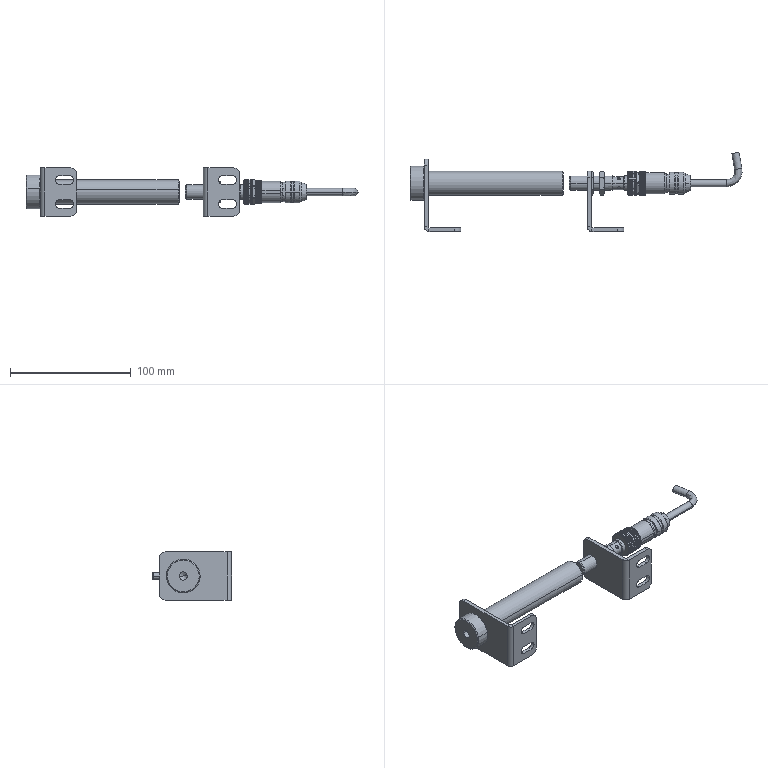Part | SolidWorks | 5 solids | 736 faces | box 275.072 x 65.521 x 40 mm | volume 76006 mm3 | plane 385 | cylinder 221 | cone 128 | spline 2 | commonest cylinder face diameters 19.5 x50 20 x40 2.5 x12 7 x12 12 x10 1 x8